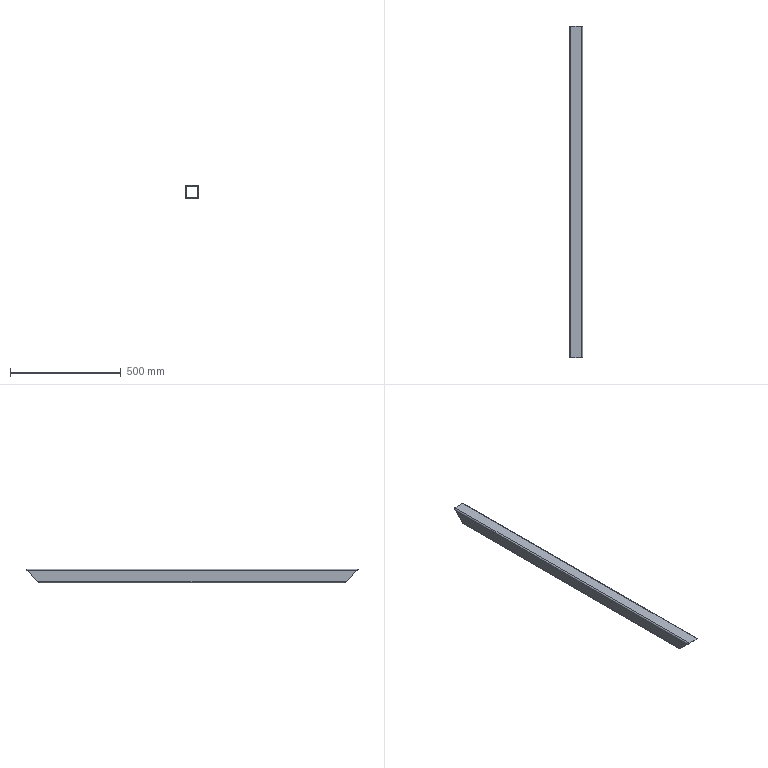Part | STEP file | Positioning_id1334_x_t | 1 solid | 14 faces | box 60 x 1500 x 60 mm | volume 1539500 mm3 | plane 10 | cylinder 4 | commonest cylinder face diameters 12 x4
STEP:
#1=CARTESIAN_POINT('',(0.,0.,0.));
#2=DIRECTION('',(0.,0.,1.));
#3=DIRECTION('',(1.,0.,0.));
#4=AXIS2_PLACEMENT_3D('',#1,#2,#3);
#5=CARTESIAN_POINT('',(-1086.002,695.,477.466));
#6=VERTEX_POINT('',#5);
#7=CARTESIAN_POINT('',(-1086.002,745.,527.466));
#8=VERTEX_POINT('',#7);
#9=CARTESIAN_POINT('',(-1086.002,695.,477.466));
#10=DIRECTION('',(0.,0.7071,0.7071));
#11=VECTOR('',#10,1.);
#12=LINE('',#9,#11);
#13=CARTESIAN_POINT('',(-1091.002,696.,478.466));
#14=DIRECTION('',(0.,-0.7071,0.7071));
#15=DIRECTION('',(0.,0.7071,0.7071));
#16=AXIS2_PLACEMENT_3D('',#13,#14,#15);
#17=PLANE('',#16);
#18=CARTESIAN_POINT('',(-1.414,-5.));
#19=DIRECTION('',(1.,0.));
#20=VECTOR('',#19,1.);
#21=LINE('',#18,#20);
#22=(GEOMETRIC_REPRESENTATION_CONTEXT(2)PARAMETRIC_REPRESENTATION_CONTEXT()REPRESENTATION_CONTEXT('',''));
#23=DEFINITIONAL_REPRESENTATION('',(#21),#22);
#24=PCURVE('',#17,#23);
#25=CARTESIAN_POINT('',(-1086.002,-375.,527.466));
#26=DIRECTION('',(-1.,0.,0.));
#27=DIRECTION('',(0.,0.,-1.));
#28=AXIS2_PLACEMENT_3D('',#25,#26,#27);
#29=PLANE('',#28);
#30=CARTESIAN_POINT('',(50.,-1070.));
#31=DIRECTION('',(-0.7071,-0.7071));
#32=VECTOR('',#31,1.);
#33=LINE('',#30,#32);
#34=(GEOMETRIC_REPRESENTATION_CONTEXT(2)PARAMETRIC_REPRESENTATION_CONTEXT()REPRESENTATION_CONTEXT('',''));
#35=DEFINITIONAL_REPRESENTATION('',(#33),#34);
#36=PCURVE('',#29,#35);
#37=SURFACE_CURVE('',#12,(#24,#36),.PCURVE_S1.);
#38=EDGE_CURVE('',#6,#8,#37,.T.);
#39=ORIENTED_EDGE('',*,*,#38,.F.);
#40=CARTESIAN_POINT('',(-1036.002,695.,477.466));
#41=VERTEX_POINT('',#40);
#42=CARTESIAN_POINT('',(-1036.002,695.,477.466));
#43=DIRECTION('',(-1.,0.,0.));
#44=VECTOR('',#43,1.);
#45=LINE('',#42,#44);
#46=CARTESIAN_POINT('',(-1.414,-55.));
#47=DIRECTION('',(0.,1.));
#48=VECTOR('',#47,1.);
#49=LINE('',#46,#48);
#50=(GEOMETRIC_REPRESENTATION_CONTEXT(2)PARAMETRIC_REPRESENTATION_CONTEXT()REPRESENTATION_CONTEXT('',''));
#51=DEFINITIONAL_REPRESENTATION('',(#49),#50);
#52=PCURVE('',#17,#51);
#53=CARTESIAN_POINT('',(-1061.002,-375.,477.466));
#54=DIRECTION('',(0.,0.,-1.));
#55=DIRECTION('',(1.,0.,0.));
#56=AXIS2_PLACEMENT_3D('',#53,#54,#55);
#57=PLANE('',#56);
#58=CARTESIAN_POINT('',(25.,-1070.));
#59=DIRECTION('',(-1.,0.));
#60=VECTOR('',#59,1.);
#61=LINE('',#58,#60);
#62=(GEOMETRIC_REPRESENTATION_CONTEXT(2)PARAMETRIC_REPRESENTATION_CONTEXT()REPRESENTATION_CONTEXT('',''));
#63=DEFINITIONAL_REPRESENTATION('',(#61),#62);
#64=PCURVE('',#57,#63);
#65=SURFACE_CURVE('',#45,(#52,#64),.PCURVE_S1.);
#66=EDGE_CURVE('',#41,#6,#65,.T.);
#67=ORIENTED_EDGE('',*,*,#66,.F.);
#68=CARTESIAN_POINT('',(-1036.002,745.,527.466));
#69=VERTEX_POINT('',#68);
#70=CARTESIAN_POINT('',(-1036.002,745.,527.466));
#71=DIRECTION('',(0.,-0.7071,-0.7071));
#72=VECTOR('',#71,1.);
#73=LINE('',#70,#72);
#74=CARTESIAN_POINT('',(69.296,-55.));
#75=DIRECTION('',(-1.,0.));
#76=VECTOR('',#75,1.);
#77=LINE('',#74,#76);
#78=(GEOMETRIC_REPRESENTATION_CONTEXT(2)PARAMETRIC_REPRESENTATION_CONTEXT()REPRESENTATION_CONTEXT('',''));
#79=DEFINITIONAL_REPRESENTATION('',(#77),#78);
#80=PCURVE('',#17,#79);
#81=CARTESIAN_POINT('',(-1036.002,-375.,527.466));
#82=DIRECTION('',(1.,0.,0.));
#83=DIRECTION('',(0.,0.,1.));
#84=AXIS2_PLACEMENT_3D('',#81,#82,#83);
#85=PLANE('',#84);
#86=CARTESIAN_POINT('',(0.,-1120.));
#87=DIRECTION('',(-0.7071,0.7071));
#88=VECTOR('',#87,1.);
#89=LINE('',#86,#88);
#90=(GEOMETRIC_REPRESENTATION_CONTEXT(2)PARAMETRIC_REPRESENTATION_CONTEXT()REPRESENTATION_CONTEXT('',''));
#91=DEFINITIONAL_REPRESENTATION('',(#89),#90);
#92=PCURVE('',#85,#91);
#93=SURFACE_CURVE('',#73,(#80,#92),.PCURVE_S1.);
#94=EDGE_CURVE('',#69,#41,#93,.T.);
#95=ORIENTED_EDGE('',*,*,#94,.F.);
#96=CARTESIAN_POINT('',(-1086.002,745.,527.466));
#97=DIRECTION('',(1.,0.,0.));
#98=VECTOR('',#97,1.);
#99=LINE('',#96,#98);
#100=CARTESIAN_POINT('',(69.296,-5.));
#101=DIRECTION('',(0.,-1.));
#102=VECTOR('',#101,1.);
#103=LINE('',#100,#102);
#104=(GEOMETRIC_REPRESENTATION_CONTEXT(2)PARAMETRIC_REPRESENTATION_CONTEXT()REPRESENTATION_CONTEXT('',''));
#105=DEFINITIONAL_REPRESENTATION('',(#103),#104);
#106=PCURVE('',#17,#105);
#107=CARTESIAN_POINT('',(-1061.002,-375.,527.466));
#108=DIRECTION('',(0.,0.,1.));
#109=DIRECTION('',(-1.,0.,0.));
#110=AXIS2_PLACEMENT_3D('',#107,#108,#109);
#111=PLANE('',#110);
#112=CARTESIAN_POINT('',(25.,-1120.));
#113=DIRECTION('',(-1.,0.));
#114=VECTOR('',#113,1.);
#115=LINE('',#112,#114);
#116=(GEOMETRIC_REPRESENTATION_CONTEXT(2)PARAMETRIC_REPRESENTATION_CONTEXT()REPRESENTATION_CONTEXT('',''));
#117=DEFINITIONAL_REPRESENTATION('',(#115),#116);
#118=PCURVE('',#111,#117);
#119=SURFACE_CURVE('',#99,(#106,#118),.PCURVE_S1.);
#120=EDGE_CURVE('',#8,#69,#119,.T.);
#121=ORIENTED_EDGE('',*,*,#120,.F.);
#122=EDGE_LOOP('',(#39,#67,#95,#121));
#123=FACE_BOUND('',#122,.T.);
#124=CARTESIAN_POINT('',(-1091.002,744.,526.466));
#125=VERTEX_POINT('',#124);
#126=CARTESIAN_POINT('',(-1085.002,750.,532.466));
#127=VERTEX_POINT('',#126);
#128=CARTESIAN_POINT('',(-1085.002,744.,526.466));
#129=DIRECTION('',(0.,0.7071,-0.7071));
#130=DIRECTION('',(0.,-0.7071,-0.7071));
#131=AXIS2_PLACEMENT_3D('',#128,#129,#130);
#132=ELLIPSE('',#131,8.485,6.);
#133=CARTESIAN_POINT('',(59.397,-6.));
#134=CARTESIAN_POINT('',(59.397,4.392));
#135=CARTESIAN_POINT('',(72.125,-0.8038));
#136=CARTESIAN_POINT('',(84.853,-6.));
#137=CARTESIAN_POINT('',(72.125,-11.196));
#138=CARTESIAN_POINT('',(59.397,-16.392));
#139=CARTESIAN_POINT('',(59.397,-6.));
#140=(BOUNDED_CURVE()B_SPLINE_CURVE(2,(#133,#134,#135,#136,#137,#138,#139),.UNSPECIFIED.,.T.,.F.)B_SPLINE_CURVE_WITH_KNOTS((1,2,2,2,2,1),(-2.094,0.,2.094,4.189,6.283,8.378),.UNSPECIFIED.)CURVE()GEOMETRIC_REPRESENTATION_ITEM()RATIONAL_B_SPLINE_CURVE((1.,0.5,1.,0.5,1.,0.5,1.))REPRESENTATION_ITEM(''));
#141=(GEOMETRIC_REPRESENTATION_CONTEXT(2)PARAMETRIC_REPRESENTATION_CONTEXT()REPRESENTATION_CONTEXT('',''));
#142=DEFINITIONAL_REPRESENTATION('',(#140),#141);
#143=PCURVE('',#17,#142);
#144=CARTESIAN_POINT('',(-1085.002,-375.,526.466));
#145=DIRECTION('',(0.,-1.,0.));
#146=DIRECTION('',(0.,0.,-1.));
#147=AXIS2_PLACEMENT_3D('',#144,#145,#146);
#148=CYLINDRICAL_SURFACE('',#147,6.);
#149=CARTESIAN_POINT('',(4.712,-1119.));
#150=CARTESIAN_POINT('',(4.689,-1119.143));
#151=CARTESIAN_POINT('',(4.641,-1119.428));
#152=CARTESIAN_POINT('',(4.57,-1119.855));
#153=CARTESIAN_POINT('',(4.498,-1120.276));
#154=CARTESIAN_POINT('',(4.427,-1120.692));
#155=CARTESIAN_POINT('',(4.355,-1121.099));
#156=CARTESIAN_POINT('',(4.284,-1121.495));
#157=CARTESIAN_POINT('',(4.213,-1121.878));
#158=CARTESIAN_POINT('',(4.141,-1122.247));
#159=CARTESIAN_POINT('',(4.07,-1122.599));
#160=CARTESIAN_POINT('',(3.998,-1122.933));
#161=CARTESIAN_POINT('',(3.927,-1123.246));
#162=CARTESIAN_POINT('',(3.856,-1123.538));
#163=CARTESIAN_POINT('',(3.784,-1123.807));
#164=CARTESIAN_POINT('',(3.713,-1124.052));
#165=CARTESIAN_POINT('',(3.641,-1124.271));
#166=CARTESIAN_POINT('',(3.57,-1124.462));
#167=CARTESIAN_POINT('',(3.499,-1124.626));
#168=CARTESIAN_POINT('',(3.427,-1124.762));
#169=CARTESIAN_POINT('',(3.356,-1124.868));
#170=CARTESIAN_POINT('',(3.284,-1124.944));
#171=CARTESIAN_POINT('',(3.213,-1124.99));
#172=CARTESIAN_POINT('',(3.165,-1125.));
#173=CARTESIAN_POINT('',(3.142,-1125.));
#174=B_SPLINE_CURVE_WITH_KNOTS('',3,(#149,#150,#151,#152,#153,#154,#155,#156,#157,#158,#159,#160,#161,#162,#163,#164,#165,#166,#167,#168,#169,#170,#171,#172,#173),.UNSPECIFIED.,.F.,.F.,(4,1,1,1,1,1,1,1,1,1,1,1,1,1,1,1,1,1,1,1,1,1,4),(1.571,1.642,1.714,1.785,1.856,1.928,1.999,2.071,2.142,2.213,2.285,2.356,2.428,2.499,2.57,2.642,2.713,2.785,2.856,2.927,2.999,3.07,3.142),.QUASI_UNIFORM_KNOTS.);
#175=(GEOMETRIC_REPRESENTATION_CONTEXT(2)PARAMETRIC_REPRESENTATION_CONTEXT()REPRESENTATION_CONTEXT('',''));
#176=DEFINITIONAL_REPRESENTATION('',(#174),#175);
#177=PCURVE('',#148,#176);
#178=SURFACE_CURVE('',#132,(#143,#177),.PCURVE_S1.);
#179=EDGE_CURVE('',#125,#127,#178,.T.);
#180=ORIENTED_EDGE('',*,*,#179,.T.);
#181=CARTESIAN_POINT('',(-1037.002,750.,532.466));
#182=VERTEX_POINT('',#181);
#183=CARTESIAN_POINT('',(-1085.002,750.,532.466));
#184=DIRECTION('',(1.,0.,0.));
#185=VECTOR('',#184,1.);
#186=LINE('',#183,#185);
#187=CARTESIAN_POINT('',(76.368,-6.));
#188=DIRECTION('',(0.,-1.));
#189=VECTOR('',#188,1.);
#190=LINE('',#187,#189);
#191=(GEOMETRIC_REPRESENTATION_CONTEXT(2)PARAMETRIC_REPRESENTATION_CONTEXT()REPRESENTATION_CONTEXT('',''));
#192=DEFINITIONAL_REPRESENTATION('',(#190),#191);
#193=PCURVE('',#17,#192);
#194=CARTESIAN_POINT('',(-1061.002,-375.,532.466));
#195=DIRECTION('',(0.,0.,1.));
#196=DIRECTION('',(-1.,0.,0.));
#197=AXIS2_PLACEMENT_3D('',#194,#195,#196);
#198=PLANE('',#197);
#199=CARTESIAN_POINT('',(24.,-1125.));
#200=DIRECTION('',(-1.,0.));
#201=VECTOR('',#200,1.);
#202=LINE('',#199,#201);
#203=(GEOMETRIC_REPRESENTATION_CONTEXT(2)PARAMETRIC_REPRESENTATION_CONTEXT()REPRESENTATION_CONTEXT('',''));
#204=DEFINITIONAL_REPRESENTATION('',(#202),#203);
#205=PCURVE('',#198,#204);
#206=SURFACE_CURVE('',#186,(#193,#205),.PCURVE_S1.);
#207=EDGE_CURVE('',#127,#182,#206,.T.);
#208=ORIENTED_EDGE('',*,*,#207,.T.);
#209=CARTESIAN_POINT('',(-1031.002,744.,526.466));
#210=VERTEX_POINT('',#209);
#211=CARTESIAN_POINT('',(-1037.002,744.,526.466));
#212=DIRECTION('',(0.,0.7071,-0.7071));
#213=DIRECTION('',(0.,0.7071,0.7071));
#214=AXIS2_PLACEMENT_3D('',#211,#212,#213);
#215=ELLIPSE('',#214,8.485,6.);
#216=CARTESIAN_POINT('',(76.368,-54.));
#217=CARTESIAN_POINT('',(76.368,-64.392));
#218=CARTESIAN_POINT('',(63.64,-59.196));
#219=CARTESIAN_POINT('',(50.912,-54.));
#220=CARTESIAN_POINT('',(63.64,-48.804));
#221=CARTESIAN_POINT('',(76.368,-43.608));
#222=CARTESIAN_POINT('',(76.368,-54.));
#223=(BOUNDED_CURVE()B_SPLINE_CURVE(2,(#216,#217,#218,#219,#220,#221,#222),.UNSPECIFIED.,.T.,.F.)B_SPLINE_CURVE_WITH_KNOTS((1,2,2,2,2,1),(-2.094,0.,2.094,4.189,6.283,8.378),.UNSPECIFIED.)CURVE()GEOMETRIC_REPRESENTATION_ITEM()RATIONAL_B_SPLINE_CURVE((1.,0.5,1.,0.5,1.,0.5,1.))REPRESENTATION_ITEM(''));
#224=(GEOMETRIC_REPRESENTATION_CONTEXT(2)PARAMETRIC_REPRESENTATION_CONTEXT()REPRESENTATION_CONTEXT('',''));
#225=DEFINITIONAL_REPRESENTATION('',(#223),#224);
#226=PCURVE('',#17,#225);
#227=CARTESIAN_POINT('',(-1037.002,-375.,526.466));
#228=DIRECTION('',(0.,1.,0.));
#229=DIRECTION('',(0.,0.,1.));
#230=AXIS2_PLACEMENT_3D('',#227,#228,#229);
#231=CYLINDRICAL_SURFACE('',#230,6.);
#232=CARTESIAN_POINT('',(0.,1125.));
#233=CARTESIAN_POINT('',(0.0238,1125.));
#234=CARTESIAN_POINT('',(0.0714,1124.99));
#235=CARTESIAN_POINT('',(0.1428,1124.944));
#236=CARTESIAN_POINT('',(0.2142,1124.868));
#237=CARTESIAN_POINT('',(0.2856,1124.762));
#238=CARTESIAN_POINT('',(0.357,1124.626));
#239=CARTESIAN_POINT('',(0.4284,1124.462));
#240=CARTESIAN_POINT('',(0.4998,1124.271));
#241=CARTESIAN_POINT('',(0.5712,1124.052));
#242=CARTESIAN_POINT('',(0.6426,1123.807));
#243=CARTESIAN_POINT('',(0.714,1123.538));
#244=CARTESIAN_POINT('',(0.7854,1123.246));
#245=CARTESIAN_POINT('',(0.8568,1122.933));
#246=CARTESIAN_POINT('',(0.9282,1122.599));
#247=CARTESIAN_POINT('',(0.9996,1122.247));
#248=CARTESIAN_POINT('',(1.071,1121.878));
#249=CARTESIAN_POINT('',(1.142,1121.495));
#250=CARTESIAN_POINT('',(1.214,1121.099));
#251=CARTESIAN_POINT('',(1.285,1120.692));
#252=CARTESIAN_POINT('',(1.357,1120.276));
#253=CARTESIAN_POINT('',(1.428,1119.855));
#254=CARTESIAN_POINT('',(1.499,1119.428));
#255=CARTESIAN_POINT('',(1.547,1119.143));
#256=CARTESIAN_POINT('',(1.571,1119.));
#257=B_SPLINE_CURVE_WITH_KNOTS('',3,(#232,#233,#234,#235,#236,#237,#238,#239,#240,#241,#242,#243,#244,#245,#246,#247,#248,#249,#250,#251,#252,#253,#254,#255,#256),.UNSPECIFIED.,.F.,.F.,(4,1,1,1,1,1,1,1,1,1,1,1,1,1,1,1,1,1,1,1,1,1,4),(0.,0.0714,0.1428,0.2142,0.2856,0.357,0.4284,0.4998,0.5712,0.6426,0.714,0.7854,0.8568,0.9282,0.9996,1.071,1.142,1.214,1.285,1.357,1.428,1.499,1.571),.QUASI_UNIFORM_KNOTS.);
#258=(GEOMETRIC_REPRESENTATION_CONTEXT(2)PARAMETRIC_REPRESENTATION_CONTEXT()REPRESENTATION_CONTEXT('',''));
#259=DEFINITIONAL_REPRESENTATION('',(#257),#258);
#260=PCURVE('',#231,#259);
#261=SURFACE_CURVE('',#215,(#226,#260),.PCURVE_S1.);
#262=EDGE_CURVE('',#182,#210,#261,.T.);
#263=ORIENTED_EDGE('',*,*,#262,.T.);
#264=CARTESIAN_POINT('',(-1031.002,696.,478.466));
#265=VERTEX_POINT('',#264);
#266=CARTESIAN_POINT('',(-1031.002,744.,526.466));
#267=DIRECTION('',(0.,-0.7071,-0.7071));
#268=VECTOR('',#267,1.);
#269=LINE('',#266,#268);
#270=CARTESIAN_POINT('',(67.882,-60.));
#271=DIRECTION('',(-1.,0.));
#272=VECTOR('',#271,1.);
#273=LINE('',#270,#272);
#274=(GEOMETRIC_REPRESENTATION_CONTEXT(2)PARAMETRIC_REPRESENTATION_CONTEXT()REPRESENTATION_CONTEXT('',''));
#275=DEFINITIONAL_REPRESENTATION('',(#273),#274);
#276=PCURVE('',#17,#275);
#277=CARTESIAN_POINT('',(-1031.002,-375.,532.466));
#278=DIRECTION('',(1.,0.,0.));
#279=DIRECTION('',(0.,0.,1.));
#280=AXIS2_PLACEMENT_3D('',#277,#278,#279);
#281=PLANE('',#280);
#282=CARTESIAN_POINT('',(-6.,-1119.));
#283=DIRECTION('',(-0.7071,0.7071));
#284=VECTOR('',#283,1.);
#285=LINE('',#282,#284);
#286=(GEOMETRIC_REPRESENTATION_CONTEXT(2)PARAMETRIC_REPRESENTATION_CONTEXT()REPRESENTATION_CONTEXT('',''));
#287=DEFINITIONAL_REPRESENTATION('',(#285),#286);
#288=PCURVE('',#281,#287);
#289=SURFACE_CURVE('',#269,(#276,#288),.PCURVE_S1.);
#290=EDGE_CURVE('',#210,#265,#289,.T.);
#291=ORIENTED_EDGE('',*,*,#290,.T.);
#292=CARTESIAN_POINT('',(-1037.002,690.,472.466));
#293=VERTEX_POINT('',#292);
#294=CARTESIAN_POINT('',(-1037.002,696.,478.466));
#295=DIRECTION('',(0.,0.7071,-0.7071));
#296=DIRECTION('',(0.,-0.7071,-0.7071));
#297=AXIS2_PLACEMENT_3D('',#294,#295,#296);
#298=ELLIPSE('',#297,8.485,6.);
#299=CARTESIAN_POINT('',(-8.485,-54.));
#300=CARTESIAN_POINT('',(-8.485,-43.608));
#301=CARTESIAN_POINT('',(4.243,-48.804));
#302=CARTESIAN_POINT('',(16.971,-54.));
#303=CARTESIAN_POINT('',(4.243,-59.196));
#304=CARTESIAN_POINT('',(-8.485,-64.392));
#305=CARTESIAN_POINT('',(-8.485,-54.));
#306=(BOUNDED_CURVE()B_SPLINE_CURVE(2,(#299,#300,#301,#302,#303,#304,#305),.UNSPECIFIED.,.T.,.F.)B_SPLINE_CURVE_WITH_KNOTS((1,2,2,2,2,1),(-2.094,0.,2.094,4.189,6.283,8.378),.UNSPECIFIED.)CURVE()GEOMETRIC_REPRESENTATION_ITEM()RATIONAL_B_SPLINE_CURVE((1.,0.5,1.,0.5,1.,0.5,1.))REPRESENTATION_ITEM(''));
#307=(GEOMETRIC_REPRESENTATION_CONTEXT(2)PARAMETRIC_REPRESENTATION_CONTEXT()REPRESENTATION_CONTEXT('',''));
#308=DEFINITIONAL_REPRESENTATION('',(#306),#307);
#309=PCURVE('',#17,#308);
#310=CARTESIAN_POINT('',(-1037.002,-375.,478.466));
#311=DIRECTION('',(0.,-1.,0.));
#312=DIRECTION('',(0.,0.,-1.));
#313=AXIS2_PLACEMENT_3D('',#310,#311,#312);
#314=CYLINDRICAL_SURFACE('',#313,6.);
#315=CARTESIAN_POINT('',(1.571,-1071.));
#316=CARTESIAN_POINT('',(1.547,-1070.857));
#317=CARTESIAN_POINT('',(1.499,-1070.572));
#318=CARTESIAN_POINT('',(1.428,-1070.145));
#319=CARTESIAN_POINT('',(1.357,-1069.724));
#320=CARTESIAN_POINT('',(1.285,-1069.308));
#321=CARTESIAN_POINT('',(1.214,-1068.901));
#322=CARTESIAN_POINT('',(1.142,-1068.505));
#323=CARTESIAN_POINT('',(1.071,-1068.122));
#324=CARTESIAN_POINT('',(0.9996,-1067.753));
#325=CARTESIAN_POINT('',(0.9282,-1067.401));
#326=CARTESIAN_POINT('',(0.8568,-1067.067));
#327=CARTESIAN_POINT('',(0.7854,-1066.754));
#328=CARTESIAN_POINT('',(0.714,-1066.462));
#329=CARTESIAN_POINT('',(0.6426,-1066.193));
#330=CARTESIAN_POINT('',(0.5712,-1065.948));
#331=CARTESIAN_POINT('',(0.4998,-1065.729));
#332=CARTESIAN_POINT('',(0.4284,-1065.538));
#333=CARTESIAN_POINT('',(0.357,-1065.374));
#334=CARTESIAN_POINT('',(0.2856,-1065.238));
#335=CARTESIAN_POINT('',(0.2142,-1065.132));
#336=CARTESIAN_POINT('',(0.1428,-1065.056));
#337=CARTESIAN_POINT('',(0.0714,-1065.01));
#338=CARTESIAN_POINT('',(0.0238,-1065.));
#339=CARTESIAN_POINT('',(0.,-1065.));
#340=B_SPLINE_CURVE_WITH_KNOTS('',3,(#315,#316,#317,#318,#319,#320,#321,#322,#323,#324,#325,#326,#327,#328,#329,#330,#331,#332,#333,#334,#335,#336,#337,#338,#339),.UNSPECIFIED.,.F.,.F.,(4,1,1,1,1,1,1,1,1,1,1,1,1,1,1,1,1,1,1,1,1,1,4),(4.712,4.784,4.855,4.927,4.998,5.069,5.141,5.212,5.284,5.355,5.426,5.498,5.569,5.641,5.712,5.783,5.855,5.926,5.998,6.069,6.14,6.212,6.283),.QUASI_UNIFORM_KNOTS.);
#341=(GEOMETRIC_REPRESENTATION_CONTEXT(2)PARAMETRIC_REPRESENTATION_CONTEXT()REPRESENTATION_CONTEXT('',''));
#342=DEFINITIONAL_REPRESENTATION('',(#340),#341);
#343=PCURVE('',#314,#342);
#344=SURFACE_CURVE('',#298,(#309,#343),.PCURVE_S1.);
#345=EDGE_CURVE('',#265,#293,#344,.T.);
#346=ORIENTED_EDGE('',*,*,#345,.T.);
#347=CARTESIAN_POINT('',(-1085.002,690.,472.466));
#348=VERTEX_POINT('',#347);
#349=CARTESIAN_POINT('',(-1037.002,690.,472.466));
#350=DIRECTION('',(-1.,0.,0.));
#351=VECTOR('',#350,1.);
#352=LINE('',#349,#351);
#353=CARTESIAN_POINT('',(-8.485,-54.));
#354=DIRECTION('',(0.,1.));
#355=VECTOR('',#354,1.);
#356=LINE('',#353,#355);
#357=(GEOMETRIC_REPRESENTATION_CONTEXT(2)PARAMETRIC_REPRESENTATION_CONTEXT()REPRESENTATION_CONTEXT('',''));
#358=DEFINITIONAL_REPRESENTATION('',(#356),#357);
#359=PCURVE('',#17,#358);
#360=CARTESIAN_POINT('',(-1061.002,-375.,472.466));
#361=DIRECTION('',(0.,0.,-1.));
#362=DIRECTION('',(1.,0.,0.));
#363=AXIS2_PLACEMENT_3D('',#360,#361,#362);
#364=PLANE('',#363);
#365=CARTESIAN_POINT('',(24.,-1065.));
#366=DIRECTION('',(-1.,0.));
#367=VECTOR('',#366,1.);
#368=LINE('',#365,#367);
#369=(GEOMETRIC_REPRESENTATION_CONTEXT(2)PARAMETRIC_REPRESENTATION_CONTEXT()REPRESENTATION_CONTEXT('',''));
#370=DEFINITIONAL_REPRESENTATION('',(#368),#369);
#371=PCURVE('',#364,#370);
#372=SURFACE_CURVE('',#352,(#359,#371),.PCURVE_S1.);
#373=EDGE_CURVE('',#293,#348,#372,.T.);
#374=ORIENTED_EDGE('',*,*,#373,.T.);
#375=CARTESIAN_POINT('',(-1091.002,696.,478.466));
#376=VERTEX_POINT('',#375);
#377=CARTESIAN_POINT('',(-1085.002,696.,478.466));
#378=DIRECTION('',(0.,0.7071,-0.7071));
#379=DIRECTION('',(0.,0.7071,0.7071));
#380=AXIS2_PLACEMENT_3D('',#377,#378,#379);
#381=ELLIPSE('',#380,8.485,6.);
#382=CARTESIAN_POINT('',(8.485,-6.));
#383=CARTESIAN_POINT('',(8.485,-16.392));
#384=CARTESIAN_POINT('',(-4.243,-11.196));
#385=CARTESIAN_POINT('',(-16.971,-6.));
#386=CARTESIAN_POINT('',(-4.243,-0.8038));
#387=CARTESIAN_POINT('',(8.485,4.392));
#388=CARTESIAN_POINT('',(8.485,-6.));
#389=(BOUNDED_CURVE()B_SPLINE_CURVE(2,(#382,#383,#384,#385,#386,#387,#388),.UNSPECIFIED.,.T.,.F.)B_SPLINE_CURVE_WITH_KNOTS((1,2,2,2,2,1),(-2.094,0.,2.094,4.189,6.283,8.378),.UNSPECIFIED.)CURVE()GEOMETRIC_REPRESENTATION_ITEM()RATIONAL_B_SPLINE_CURVE((1.,0.5,1.,0.5,1.,0.5,1.))REPRESENTATION_ITEM(''));
#390=(GEOMETRIC_REPRESENTATION_CONTEXT(2)PARAMETRIC_REPRESENTATION_CONTEXT()REPRESENTATION_CONTEXT('',''));
#391=DEFINITIONAL_REPRESENTATION('',(#389),#390);
#392=PCURVE('',#17,#391);
#393=CARTESIAN_POINT('',(-1085.002,-375.,478.466));
#394=DIRECTION('',(0.,1.,0.));
#395=DIRECTION('',(0.,0.,1.));
#396=AXIS2_PLACEMENT_3D('',#393,#394,#395);
#397=CYLINDRICAL_SURFACE('',#396,6.);
#398=CARTESIAN_POINT('',(3.142,1065.));
#399=CARTESIAN_POINT('',(3.165,1065.));
#400=CARTESIAN_POINT('',(3.213,1065.01));
#401=CARTESIAN_POINT('',(3.284,1065.056));
#402=CARTESIAN_POINT('',(3.356,1065.132));
#403=CARTESIAN_POINT('',(3.427,1065.238));
#404=CARTESIAN_POINT('',(3.499,1065.374));
#405=CARTESIAN_POINT('',(3.57,1065.538));
#406=CARTESIAN_POINT('',(3.641,1065.729));
#407=CARTESIAN_POINT('',(3.713,1065.948));
#408=CARTESIAN_POINT('',(3.784,1066.193));
#409=CARTESIAN_POINT('',(3.856,1066.462));
#410=CARTESIAN_POINT('',(3.927,1066.754));
#411=CARTESIAN_POINT('',(3.998,1067.067));
#412=CARTESIAN_POINT('',(4.07,1067.401));
#413=CARTESIAN_POINT('',(4.141,1067.753));
#414=CARTESIAN_POINT('',(4.213,1068.122));
#415=CARTESIAN_POINT('',(4.284,1068.505));
#416=CARTESIAN_POINT('',(4.355,1068.901));
#417=CARTESIAN_POINT('',(4.427,1069.308));
#418=CARTESIAN_POINT('',(4.498,1069.724));
#419=CARTESIAN_POINT('',(4.57,1070.145));
#420=CARTESIAN_POINT('',(4.641,1070.572));
#421=CARTESIAN_POINT('',(4.689,1070.857));
#422=CARTESIAN_POINT('',(4.712,1071.));
#423=B_SPLINE_CURVE_WITH_KNOTS('',3,(#398,#399,#400,#401,#402,#403,#404,#405,#406,#407,#408,#409,#410,#411,#412,#413,#414,#415,#416,#417,#418,#419,#420,#421,#422),.UNSPECIFIED.,.F.,.F.,(4,1,1,1,1,1,1,1,1,1,1,1,1,1,1,1,1,1,1,1,1,1,4),(3.142,3.213,3.284,3.356,3.427,3.499,3.57,3.641,3.713,3.784,3.856,3.927,3.998,4.07,4.141,4.213,4.284,4.355,4.427,4.498,4.57,4.641,4.712),.QUASI_UNIFORM_KNOTS.);
#424=(GEOMETRIC_REPRESENTATION_CONTEXT(2)PARAMETRIC_REPRESENTATION_CONTEXT()REPRESENTATION_CONTEXT('',''));
#425=DEFINITIONAL_REPRESENTATION('',(#423),#424);
#426=PCURVE('',#397,#425);
#427=SURFACE_CURVE('',#381,(#392,#426),.PCURVE_S1.);
#428=EDGE_CURVE('',#348,#376,#427,.T.);
#429=ORIENTED_EDGE('',*,*,#428,.T.);
#430=CARTESIAN_POINT('',(-1091.002,696.,478.466));
#431=DIRECTION('',(0.,0.7071,0.7071));
#432=VECTOR('',#431,1.);
#433=LINE('',#430,#432);
#434=CARTESIAN_POINT('',(0.,0.));
#435=DIRECTION('',(1.,0.));
#436=VECTOR('',#435,1.);
#437=LINE('',#434,#436);
#438=(GEOMETRIC_REPRESENTATION_CONTEXT(2)PARAMETRIC_REPRESENTATION_CONTEXT()REPRESENTATION_CONTEXT('',''));
#439=DEFINITIONAL_REPRESENTATION('',(#437),#438);
#440=PCURVE('',#17,#439);
#441=CARTESIAN_POINT('',(-1091.002,-375.,532.466));
#442=DIRECTION('',(-1.,0.,0.));
#443=DIRECTION('',(0.,0.,-1.));
#444=AXIS2_PLACEMENT_3D('',#441,#442,#443);
#445=PLANE('',#444);
#446=CARTESIAN_POINT('',(54.,-1071.));
#447=DIRECTION('',(-0.7071,-0.7071));
#448=VECTOR('',#447,1.);
#449=LINE('',#446,#448);
#450=(GEOMETRIC_REPRESENTATION_CONTEXT(2)PARAMETRIC_REPRESENTATION_CONTEXT()REPRESENTATION_CONTEXT('',''));
#451=DEFINITIONAL_REPRESENTATION('',(#449),#450);
#452=PCURVE('',#445,#451);
#453=SURFACE_CURVE('',#433,(#440,#452),.PCURVE_S1.);
#454=EDGE_CURVE('',#376,#125,#453,.T.);
#455=ORIENTED_EDGE('',*,*,#454,.T.);
#456=EDGE_LOOP('',(#180,#208,#263,#291,#346,#374,#429,#455));
#457=FACE_BOUND('',#456,.T.);
#458=ADVANCED_FACE('',(#123,#457),#17,.F.);
#459=CARTESIAN_POINT('',(-1036.002,-695.,477.466));
#460=VERTEX_POINT('',#459);
#461=CARTESIAN_POINT('',(-1086.002,-695.,477.466));
#462=VERTEX_POINT('',#461);
#463=CARTESIAN_POINT('',(-1036.002,-695.,477.466));
#464=DIRECTION('',(-1.,0.,0.));
#465=VECTOR('',#464,1.);
#466=LINE('',#463,#465);
#467=CARTESIAN_POINT('',(-1091.002,-696.,478.466));
#468=DIRECTION('',(0.,-0.7071,-0.7071));
#469=DIRECTION('',(0.,-0.7071,0.7071));
#470=AXIS2_PLACEMENT_3D('',#467,#468,#469);
#471=PLANE('',#470);
#472=CARTESIAN_POINT('',(-1.414,-55.));
#473=DIRECTION('',(0.,1.));
#474=VECTOR('',#473,1.);
#475=LINE('',#472,#474);
#476=(GEOMETRIC_REPRESENTATION_CONTEXT(2)PARAMETRIC_REPRESENTATION_CONTEXT()REPRESENTATION_CONTEXT('',''));
#477=DEFINITIONAL_REPRESENTATION('',(#475),#476);
#478=PCURVE('',#471,#477);
#479=CARTESIAN_POINT('',(25.,320.));
#480=DIRECTION('',(-1.,0.));
#481=VECTOR('',#480,1.);
#482=LINE('',#479,#481);
#483=(GEOMETRIC_REPRESENTATION_CONTEXT(2)PARAMETRIC_REPRESENTATION_CONTEXT()REPRESENTATION_CONTEXT('',''));
#484=DEFINITIONAL_REPRESENTATION('',(#482),#483);
#485=PCURVE('',#57,#484);
#486=SURFACE_CURVE('',#466,(#478,#485),.PCURVE_S1.);
#487=EDGE_CURVE('',#460,#462,#486,.T.);
#488=ORIENTED_EDGE('',*,*,#487,.T.);
#489=CARTESIAN_POINT('',(-1086.002,-745.,527.466));
#490=VERTEX_POINT('',#489);
#491=CARTESIAN_POINT('',(-1086.002,-695.,477.466));
#492=DIRECTION('',(0.,-0.7071,0.7071));
#493=VECTOR('',#492,1.);
#494=LINE('',#491,#493);
#495=CARTESIAN_POINT('',(-1.414,-5.));
#496=DIRECTION('',(1.,0.));
#497=VECTOR('',#496,1.);
#498=LINE('',#495,#497);
#499=(GEOMETRIC_REPRESENTATION_CONTEXT(2)PARAMETRIC_REPRESENTATION_CONTEXT()REPRESENTATION_CONTEXT('',''));
#500=DEFINITIONAL_REPRESENTATION('',(#498),#499);
#501=PCURVE('',#471,#500);
#502=CARTESIAN_POINT('',(50.,320.));
#503=DIRECTION('',(-0.7071,0.7071));
#504=VECTOR('',#503,1.);
#505=LINE('',#502,#504);
#506=(GEOMETRIC_REPRESENTATION_CONTEXT(2)PARAMETRIC_REPRESENTATION_CONTEXT()REPRESENTATION_CONTEXT('',''));
#507=DEFINITIONAL_REPRESENTATION('',(#505),#506);
#508=PCURVE('',#29,#507);
#509=SURFACE_CURVE('',#494,(#501,#508),.PCURVE_S1.);
#510=EDGE_CURVE('',#462,#490,#509,.T.);
#511=ORIENTED_EDGE('',*,*,#510,.T.);
#512=CARTESIAN_POINT('',(-1036.002,-745.,527.466));
#513=VERTEX_POINT('',#512);
#514=CARTESIAN_POINT('',(-1086.002,-745.,527.466));
#515=DIRECTION('',(1.,0.,0.));
#516=VECTOR('',#515,1.);
#517=LINE('',#514,#516);
#518=CARTESIAN_POINT('',(69.296,-5.));
#519=DIRECTION('',(0.,-1.));
#520=VECTOR('',#519,1.);
#521=LINE('',#518,#520);
#522=(GEOMETRIC_REPRESENTATION_CONTEXT(2)PARAMETRIC_REPRESENTATION_CONTEXT()REPRESENTATION_CONTEXT('',''));
#523=DEFINITIONAL_REPRESENTATION('',(#521),#522);
#524=PCURVE('',#471,#523);
#525=CARTESIAN_POINT('',(25.,370.));
#526=DIRECTION('',(-1.,0.));
#527=VECTOR('',#526,1.);
#528=LINE('',#525,#527);
#529=(GEOMETRIC_REPRESENTATION_CONTEXT(2)PARAMETRIC_REPRESENTATION_CONTEXT()REPRESENTATION_CONTEXT('',''));
#530=DEFINITIONAL_REPRESENTATION('',(#528),#529);
#531=PCURVE('',#111,#530);
#532=SURFACE_CURVE('',#517,(#524,#531),.PCURVE_S1.);
#533=EDGE_CURVE('',#490,#513,#532,.T.);
#534=ORIENTED_EDGE('',*,*,#533,.T.);
#535=CARTESIAN_POINT('',(-1036.002,-745.,527.466));
#536=DIRECTION('',(0.,0.7071,-0.7071));
#537=VECTOR('',#536,1.);
#538=LINE('',#535,#537);
#539=CARTESIAN_POINT('',(69.296,-55.));
#540=DIRECTION('',(-1.,0.));
#541=VECTOR('',#540,1.);
#542=LINE('',#539,#541);
#543=(GEOMETRIC_REPRESENTATION_CONTEXT(2)PARAMETRIC_REPRESENTATION_CONTEXT()REPRESENTATION_CONTEXT('',''));
#544=DEFINITIONAL_REPRESENTATION('',(#542),#543);
#545=PCURVE('',#471,#544);
#546=CARTESIAN_POINT('',(0.,370.));
#547=DIRECTION('',(-0.7071,-0.7071));
#548=VECTOR('',#547,1.);
#549=LINE('',#546,#548);
#550=(GEOMETRIC_REPRESENTATION_CONTEXT(2)PARAMETRIC_REPRESENTATION_CONTEXT()REPRESENTATION_CONTEXT('',''));
#551=DEFINITIONAL_REPRESENTATION('',(#549),#550);
#552=PCURVE('',#85,#551);
#553=SURFACE_CURVE('',#538,(#545,#552),.PCURVE_S1.);
#554=EDGE_CURVE('',#513,#460,#553,.T.);
#555=ORIENTED_EDGE('',*,*,#554,.T.);
#556=EDGE_LOOP('',(#488,#511,#534,#555));
#557=FACE_BOUND('',#556,.T.);
#558=CARTESIAN_POINT('',(-1085.002,-750.,532.466));
#559=VERTEX_POINT('',#558);
#560=CARTESIAN_POINT('',(-1037.002,-750.,532.466));
#561=VERTEX_POINT('',#560);
#562=CARTESIAN_POINT('',(-1085.002,-750.,532.466));
#563=DIRECTION('',(1.,0.,0.));
#564=VECTOR('',#563,1.);
#565=LINE('',#562,#564);
#566=CARTESIAN_POINT('',(76.368,-6.));
#567=DIRECTION('',(0.,-1.));
#568=VECTOR('',#567,1.);
#569=LINE('',#566,#568);
#570=(GEOMETRIC_REPRESENTATION_CONTEXT(2)PARAMETRIC_REPRESENTATION_CONTEXT()REPRESENTATION_CONTEXT('',''));
#571=DEFINITIONAL_REPRESENTATION('',(#569),#570);
#572=PCURVE('',#471,#571);
#573=CARTESIAN_POINT('',(24.,375.));
#574=DIRECTION('',(-1.,0.));
#575=VECTOR('',#574,1.);
#576=LINE('',#573,#575);
#577=(GEOMETRIC_REPRESENTATION_CONTEXT(2)PARAMETRIC_REPRESENTATION_CONTEXT()REPRESENTATION_CONTEXT('',''));
#578=DEFINITIONAL_REPRESENTATION('',(#576),#577);
#579=PCURVE('',#198,#578);
#580=SURFACE_CURVE('',#565,(#572,#579),.PCURVE_S1.);
#581=EDGE_CURVE('',#559,#561,#580,.T.);
#582=ORIENTED_EDGE('',*,*,#581,.F.);
#583=CARTESIAN_POINT('',(-1091.002,-744.,526.466));
#584=VERTEX_POINT('',#583);
#585=CARTESIAN_POINT('',(-1085.002,-744.,526.466));
#586=DIRECTION('',(0.,0.7071,0.7071));
#587=DIRECTION('',(0.,-0.7071,0.7071));
#588=AXIS2_PLACEMENT_3D('',#585,#586,#587);
#589=ELLIPSE('',#588,8.485,6.);
#590=CARTESIAN_POINT('',(76.368,-6.));
#591=CARTESIAN_POINT('',(76.368,-16.392));
#592=CARTESIAN_POINT('',(63.64,-11.196));
#593=CARTESIAN_POINT('',(50.912,-6.));
#594=CARTESIAN_POINT('',(63.64,-0.8038));
#595=CARTESIAN_POINT('',(76.368,4.392));
#596=CARTESIAN_POINT('',(76.368,-6.));
#597=(BOUNDED_CURVE()B_SPLINE_CURVE(2,(#590,#591,#592,#593,#594,#595,#596),.UNSPECIFIED.,.T.,.F.)B_SPLINE_CURVE_WITH_KNOTS((1,2,2,2,2,1),(-2.094,0.,2.094,4.189,6.283,8.378),.UNSPECIFIED.)CURVE()GEOMETRIC_REPRESENTATION_ITEM()RATIONAL_B_SPLINE_CURVE((1.,0.5,1.,0.5,1.,0.5,1.))REPRESENTATION_ITEM(''));
#598=(GEOMETRIC_REPRESENTATION_CONTEXT(2)PARAMETRIC_REPRESENTATION_CONTEXT()REPRESENTATION_CONTEXT('',''));
#599=DEFINITIONAL_REPRESENTATION('',(#597),#598);
#600=PCURVE('',#471,#599);
#601=CARTESIAN_POINT('',(4.712,369.));
#602=CARTESIAN_POINT('',(4.689,369.143));
#603=CARTESIAN_POINT('',(4.641,369.428));
#604=CARTESIAN_POINT('',(4.57,369.855));
#605=CARTESIAN_POINT('',(4.498,370.276));
#606=CARTESIAN_POINT('',(4.427,370.692));
#607=CARTESIAN_POINT('',(4.355,371.099));
#608=CARTESIAN_POINT('',(4.284,371.495));
#609=CARTESIAN_POINT('',(4.213,371.878));
#610=CARTESIAN_POINT('',(4.141,372.247));
#611=CARTESIAN_POINT('',(4.07,372.599));
#612=CARTESIAN_POINT('',(3.998,372.933));
#613=CARTESIAN_POINT('',(3.927,373.246));
#614=CARTESIAN_POINT('',(3.856,373.538));
#615=CARTESIAN_POINT('',(3.784,373.807));
#616=CARTESIAN_POINT('',(3.713,374.052));
#617=CARTESIAN_POINT('',(3.641,374.271));
#618=CARTESIAN_POINT('',(3.57,374.462));
#619=CARTESIAN_POINT('',(3.499,374.626));
#620=CARTESIAN_POINT('',(3.427,374.762));
#621=CARTESIAN_POINT('',(3.356,374.868));
#622=CARTESIAN_POINT('',(3.284,374.944));
#623=CARTESIAN_POINT('',(3.213,374.99));
#624=CARTESIAN_POINT('',(3.165,375.));
#625=CARTESIAN_POINT('',(3.142,375.));
#626=B_SPLINE_CURVE_WITH_KNOTS('',3,(#601,#602,#603,#604,#605,#606,#607,#608,#609,#610,#611,#612,#613,#614,#615,#616,#617,#618,#619,#620,#621,#622,#623,#624,#625),.UNSPECIFIED.,.F.,.F.,(4,1,1,1,1,1,1,1,1,1,1,1,1,1,1,1,1,1,1,1,1,1,4),(4.712,4.784,4.855,4.927,4.998,5.069,5.141,5.212,5.284,5.355,5.426,5.498,5.569,5.641,5.712,5.783,5.855,5.926,5.998,6.069,6.14,6.212,6.283),.QUASI_UNIFORM_KNOTS.);
#627=(GEOMETRIC_REPRESENTATION_CONTEXT(2)PARAMETRIC_REPRESENTATION_CONTEXT()REPRESENTATION_CONTEXT('',''));
#628=DEFINITIONAL_REPRESENTATION('',(#626),#627);
#629=PCURVE('',#148,#628);
#630=SURFACE_CURVE('',#589,(#600,#629),.PCURVE_S1.);
#631=EDGE_CURVE('',#584,#559,#630,.T.);
#632=ORIENTED_EDGE('',*,*,#631,.F.);
#633=CARTESIAN_POINT('',(-1091.002,-696.,478.466));
#634=VERTEX_POINT('',#633);
#635=CARTESIAN_POINT('',(-1091.002,-696.,478.466));
#636=DIRECTION('',(0.,-0.7071,0.7071));
#637=VECTOR('',#636,1.);
#638=LINE('',#635,#637);
#639=CARTESIAN_POINT('',(0.,0.));
#640=DIRECTION('',(1.,0.));
#641=VECTOR('',#640,1.);
#642=LINE('',#639,#641);
#643=(GEOMETRIC_REPRESENTATION_CONTEXT(2)PARAMETRIC_REPRESENTATION_CONTEXT()REPRESENTATION_CONTEXT('',''));
#644=DEFINITIONAL_REPRESENTATION('',(#642),#643);
#645=PCURVE('',#471,#644);
#646=CARTESIAN_POINT('',(54.,321.));
#647=DIRECTION('',(-0.7071,0.7071));
#648=VECTOR('',#647,1.);
#649=LINE('',#646,#648);
#650=(GEOMETRIC_REPRESENTATION_CONTEXT(2)PARAMETRIC_REPRESENTATION_CONTEXT()REPRESENTATION_CONTEXT('',''));
#651=DEFINITIONAL_REPRESENTATION('',(#649),#650);
#652=PCURVE('',#445,#651);
#653=SURFACE_CURVE('',#638,(#645,#652),.PCURVE_S1.);
#654=EDGE_CURVE('',#634,#584,#653,.T.);
#655=ORIENTED_EDGE('',*,*,#654,.F.);
#656=CARTESIAN_POINT('',(-1085.002,-690.,472.466));
#657=VERTEX_POINT('',#656);
#658=CARTESIAN_POINT('',(-1085.002,-696.,478.466));
#659=DIRECTION('',(0.,0.7071,0.7071));
#660=DIRECTION('',(0.,0.7071,-0.7071));
#661=AXIS2_PLACEMENT_3D('',#658,#659,#660);
#662=ELLIPSE('',#661,8.485,6.);
#663=CARTESIAN_POINT('',(-8.485,-6.));
#664=CARTESIAN_POINT('',(-8.485,4.392));
#665=CARTESIAN_POINT('',(4.243,-0.8038));
#666=CARTESIAN_POINT('',(16.971,-6.));
#667=CARTESIAN_POINT('',(4.243,-11.196));
#668=CARTESIAN_POINT('',(-8.485,-16.392));
#669=CARTESIAN_POINT('',(-8.485,-6.));
#670=(BOUNDED_CURVE()B_SPLINE_CURVE(2,(#663,#664,#665,#666,#667,#668,#669),.UNSPECIFIED.,.T.,.F.)B_SPLINE_CURVE_WITH_KNOTS((1,2,2,2,2,1),(-2.094,0.,2.094,4.189,6.283,8.378),.UNSPECIFIED.)CURVE()GEOMETRIC_REPRESENTATION_ITEM()RATIONAL_B_SPLINE_CURVE((1.,0.5,1.,0.5,1.,0.5,1.))REPRESENTATION_ITEM(''));
#671=(GEOMETRIC_REPRESENTATION_CONTEXT(2)PARAMETRIC_REPRESENTATION_CONTEXT()REPRESENTATION_CONTEXT('',''));
#672=DEFINITIONAL_REPRESENTATION('',(#670),#671);
#673=PCURVE('',#471,#672);
#674=CARTESIAN_POINT('',(3.142,-315.));
#675=CARTESIAN_POINT('',(3.165,-315.));
#676=CARTESIAN_POINT('',(3.213,-315.01));
#677=CARTESIAN_POINT('',(3.284,-315.056));
#678=CARTESIAN_POINT('',(3.356,-315.132));
#679=CARTESIAN_POINT('',(3.427,-315.238));
#680=CARTESIAN_POINT('',(3.499,-315.374));
#681=CARTESIAN_POINT('',(3.57,-315.538));
#682=CARTESIAN_POINT('',(3.641,-315.729));
#683=CARTESIAN_POINT('',(3.713,-315.948));
#684=CARTESIAN_POINT('',(3.784,-316.193));
#685=CARTESIAN_POINT('',(3.856,-316.462));
#686=CARTESIAN_POINT('',(3.927,-316.754));
#687=CARTESIAN_POINT('',(3.998,-317.067));
#688=CARTESIAN_POINT('',(4.07,-317.401));
#689=CARTESIAN_POINT('',(4.141,-317.753));
#690=CARTESIAN_POINT('',(4.213,-318.122));
#691=CARTESIAN_POINT('',(4.284,-318.505));
#692=CARTESIAN_POINT('',(4.355,-318.901));
#693=CARTESIAN_POINT('',(4.427,-319.308));
#694=CARTESIAN_POINT('',(4.498,-319.724));
#695=CARTESIAN_POINT('',(4.57,-320.145));
#696=CARTESIAN_POINT('',(4.641,-320.572));
#697=CARTESIAN_POINT('',(4.689,-320.857));
#698=CARTESIAN_POINT('',(4.712,-321.));
#699=B_SPLINE_CURVE_WITH_KNOTS('',3,(#674,#675,#676,#677,#678,#679,#680,#681,#682,#683,#684,#685,#686,#687,#688,#689,#690,#691,#692,#693,#694,#695,#696,#697,#698),.UNSPECIFIED.,.F.,.F.,(4,1,1,1,1,1,1,1,1,1,1,1,1,1,1,1,1,1,1,1,1,1,4),(0.,0.0714,0.1428,0.2142,0.2856,0.357,0.4284,0.4998,0.5712,0.6426,0.714,0.7854,0.8568,0.9282,0.9996,1.071,1.142,1.214,1.285,1.357,1.428,1.499,1.571),.QUASI_UNIFORM_KNOTS.);
#700=(GEOMETRIC_REPRESENTATION_CONTEXT(2)PARAMETRIC_REPRESENTATION_CONTEXT()REPRESENTATION_CONTEXT('',''));
#701=DEFINITIONAL_REPRESENTATION('',(#699),#700);
#702=PCURVE('',#397,#701);
#703=SURFACE_CURVE('',#662,(#673,#702),.PCURVE_S1.);
#704=EDGE_CURVE('',#657,#634,#703,.T.);
#705=ORIENTED_EDGE('',*,*,#704,.F.);
#706=CARTESIAN_POINT('',(-1037.002,-690.,472.466));
#707=VERTEX_POINT('',#706);
#708=CARTESIAN_POINT('',(-1037.002,-690.,472.466));
#709=DIRECTION('',(-1.,0.,0.));
#710=VECTOR('',#709,1.);
#711=LINE('',#708,#710);
#712=CARTESIAN_POINT('',(-8.485,-54.));
#713=DIRECTION('',(0.,1.));
#714=VECTOR('',#713,1.);
#715=LINE('',#712,#714);
#716=(GEOMETRIC_REPRESENTATION_CONTEXT(2)PARAMETRIC_REPRESENTATION_CONTEXT()REPRESENTATION_CONTEXT('',''));
#717=DEFINITIONAL_REPRESENTATION('',(#715),#716);
#718=PCURVE('',#471,#717);
#719=CARTESIAN_POINT('',(24.,315.));
#720=DIRECTION('',(-1.,0.));
#721=VECTOR('',#720,1.);
#722=LINE('',#719,#721);
#723=(GEOMETRIC_REPRESENTATION_CONTEXT(2)PARAMETRIC_REPRESENTATION_CONTEXT()REPRESENTATION_CONTEXT('',''));
#724=DEFINITIONAL_REPRESENTATION('',(#722),#723);
#725=PCURVE('',#364,#724);
#726=SURFACE_CURVE('',#711,(#718,#725),.PCURVE_S1.);
#727=EDGE_CURVE('',#707,#657,#726,.T.);
#728=ORIENTED_EDGE('',*,*,#727,.F.);
#729=CARTESIAN_POINT('',(-1031.002,-696.,478.466));
#730=VERTEX_POINT('',#729);
#731=CARTESIAN_POINT('',(-1037.002,-696.,478.466));
#732=DIRECTION('',(0.,0.7071,0.7071));
#733=DIRECTION('',(0.,-0.7071,0.7071));
#734=AXIS2_PLACEMENT_3D('',#731,#732,#733);
#735=ELLIPSE('',#734,8.485,6.);
#736=CARTESIAN_POINT('',(8.485,-54.));
#737=CARTESIAN_POINT('',(8.485,-64.392));
#738=CARTESIAN_POINT('',(-4.243,-59.196));
#739=CARTESIAN_POINT('',(-16.971,-54.));
#740=CARTESIAN_POINT('',(-4.243,-48.804));
#741=CARTESIAN_POINT('',(8.485,-43.608));
#742=CARTESIAN_POINT('',(8.485,-54.));
#743=(BOUNDED_CURVE()B_SPLINE_CURVE(2,(#736,#737,#738,#739,#740,#741,#742),.UNSPECIFIED.,.T.,.F.)B_SPLINE_CURVE_WITH_KNOTS((1,2,2,2,2,1),(-2.094,0.,2.094,4.189,6.283,8.378),.UNSPECIFIED.)CURVE()GEOMETRIC_REPRESENTATION_ITEM()RATIONAL_B_SPLINE_CURVE((1.,0.5,1.,0.5,1.,0.5,1.))REPRESENTATION_ITEM(''));
#744=(GEOMETRIC_REPRESENTATION_CONTEXT(2)PARAMETRIC_REPRESENTATION_CONTEXT()REPRESENTATION_CONTEXT('',''));
#745=DEFINITIONAL_REPRESENTATION('',(#743),#744);
#746=PCURVE('',#471,#745);
#747=CARTESIAN_POINT('',(1.571,321.));
#748=CARTESIAN_POINT('',(1.547,320.857));
#749=CARTESIAN_POINT('',(1.499,320.572));
#750=CARTESIAN_POINT('',(1.428,320.145));
#751=CARTESIAN_POINT('',(1.357,319.724));
#752=CARTESIAN_POINT('',(1.285,319.308));
#753=CARTESIAN_POINT('',(1.214,318.901));
#754=CARTESIAN_POINT('',(1.142,318.505));
#755=CARTESIAN_POINT('',(1.071,318.122));
#756=CARTESIAN_POINT('',(0.9996,317.753));
#757=CARTESIAN_POINT('',(0.9282,317.401));
#758=CARTESIAN_POINT('',(0.8568,317.067));
#759=CARTESIAN_POINT('',(0.7854,316.754));
#760=CARTESIAN_POINT('',(0.714,316.462));
#761=CARTESIAN_POINT('',(0.6426,316.193));
#762=CARTESIAN_POINT('',(0.5712,315.948));
#763=CARTESIAN_POINT('',(0.4998,315.729));
#764=CARTESIAN_POINT('',(0.4284,315.538));
#765=CARTESIAN_POINT('',(0.357,315.374));
#766=CARTESIAN_POINT('',(0.2856,315.238));
#767=CARTESIAN_POINT('',(0.2142,315.132));
#768=CARTESIAN_POINT('',(0.1428,315.056));
#769=CARTESIAN_POINT('',(0.0714,315.01));
#770=CARTESIAN_POINT('',(0.0238,315.));
#771=CARTESIAN_POINT('',(0.,315.));
#772=B_SPLINE_CURVE_WITH_KNOTS('',3,(#747,#748,#749,#750,#751,#752,#753,#754,#755,#756,#757,#758,#759,#760,#761,#762,#763,#764,#765,#766,#767,#768,#769,#770,#771),.UNSPECIFIED.,.F.,.F.,(4,1,1,1,1,1,1,1,1,1,1,1,1,1,1,1,1,1,1,1,1,1,4),(1.571,1.642,1.714,1.785,1.856,1.928,1.999,2.071,2.142,2.213,2.285,2.356,2.428,2.499,2.57,2.642,2.713,2.785,2.856,2.927,2.999,3.07,3.142),.QUASI_UNIFORM_KNOTS.);
#773=(GEOMETRIC_REPRESENTATION_CONTEXT(2)PARAMETRIC_REPRESENTATION_CONTEXT()REPRESENTATION_CONTEXT('',''));
#774=DEFINITIONAL_REPRESENTATION('',(#772),#773);
#775=PCURVE('',#314,#774);
#776=SURFACE_CURVE('',#735,(#746,#775),.PCURVE_S1.);
#777=EDGE_CURVE('',#730,#707,#776,.T.);
#778=ORIENTED_EDGE('',*,*,#777,.F.);
#779=CARTESIAN_POINT('',(-1031.002,-744.,526.466));
#780=VERTEX_POINT('',#779);
#781=CARTESIAN_POINT('',(-1031.002,-744.,526.466));
#782=DIRECTION('',(0.,0.7071,-0.7071));
#783=VECTOR('',#782,1.);
#784=LINE('',#781,#783);
#785=CARTESIAN_POINT('',(67.882,-60.));
#786=DIRECTION('',(-1.,0.));
#787=VECTOR('',#786,1.);
#788=LINE('',#785,#787);
#789=(GEOMETRIC_REPRESENTATION_CONTEXT(2)PARAMETRIC_REPRESENTATION_CONTEXT()REPRESENTATION_CONTEXT('',''));
#790=DEFINITIONAL_REPRESENTATION('',(#788),#789);
#791=PCURVE('',#471,#790);
#792=CARTESIAN_POINT('',(-6.,369.));
#793=DIRECTION('',(-0.7071,-0.7071));
#794=VECTOR('',#793,1.);
#795=LINE('',#792,#794);
#796=(GEOMETRIC_REPRESENTATION_CONTEXT(2)PARAMETRIC_REPRESENTATION_CONTEXT()REPRESENTATION_CONTEXT('',''));
#797=DEFINITIONAL_REPRESENTATION('',(#795),#796);
#798=PCURVE('',#281,#797);
#799=SURFACE_CURVE('',#784,(#791,#798),.PCURVE_S1.);
#800=EDGE_CURVE('',#780,#730,#799,.T.);
#801=ORIENTED_EDGE('',*,*,#800,.F.);
#802=CARTESIAN_POINT('',(-1037.002,-744.,526.466));
#803=DIRECTION('',(0.,0.7071,0.7071));
#804=DIRECTION('',(0.,0.7071,-0.7071));
#805=AXIS2_PLACEMENT_3D('',#802,#803,#804);
#806=ELLIPSE('',#805,8.485,6.);
#807=CARTESIAN_POINT('',(59.397,-54.));
#808=CARTESIAN_POINT('',(59.397,-43.608));
#809=CARTESIAN_POINT('',(72.125,-48.804));
#810=CARTESIAN_POINT('',(84.853,-54.));
#811=CARTESIAN_POINT('',(72.125,-59.196));
#812=CARTESIAN_POINT('',(59.397,-64.392));
#813=CARTESIAN_POINT('',(59.397,-54.));
#814=(BOUNDED_CURVE()B_SPLINE_CURVE(2,(#807,#808,#809,#810,#811,#812,#813),.UNSPECIFIED.,.T.,.F.)B_SPLINE_CURVE_WITH_KNOTS((1,2,2,2,2,1),(-2.094,0.,2.094,4.189,6.283,8.378),.UNSPECIFIED.)CURVE()GEOMETRIC_REPRESENTATION_ITEM()RATIONAL_B_SPLINE_CURVE((1.,0.5,1.,0.5,1.,0.5,1.))REPRESENTATION_ITEM(''));
#815=(GEOMETRIC_REPRESENTATION_CONTEXT(2)PARAMETRIC_REPRESENTATION_CONTEXT()REPRESENTATION_CONTEXT('',''));
#816=DEFINITIONAL_REPRESENTATION('',(#814),#815);
#817=PCURVE('',#471,#816);
#818=CARTESIAN_POINT('',(0.,-375.));
#819=CARTESIAN_POINT('',(0.0238,-375.));
#820=CARTESIAN_POINT('',(0.0714,-374.99));
#821=CARTESIAN_POINT('',(0.1428,-374.944));
#822=CARTESIAN_POINT('',(0.2142,-374.868));
#823=CARTESIAN_POINT('',(0.2856,-374.762));
#824=CARTESIAN_POINT('',(0.357,-374.626));
#825=CARTESIAN_POINT('',(0.4284,-374.462));
#826=CARTESIAN_POINT('',(0.4998,-374.271));
#827=CARTESIAN_POINT('',(0.5712,-374.052));
#828=CARTESIAN_POINT('',(0.6426,-373.807));
#829=CARTESIAN_POINT('',(0.714,-373.538));
#830=CARTESIAN_POINT('',(0.7854,-373.246));
#831=CARTESIAN_POINT('',(0.8568,-372.933));
#832=CARTESIAN_POINT('',(0.9282,-372.599));
#833=CARTESIAN_POINT('',(0.9996,-372.247));
#834=CARTESIAN_POINT('',(1.071,-371.878));
#835=CARTESIAN_POINT('',(1.142,-371.495));
#836=CARTESIAN_POINT('',(1.214,-371.099));
#837=CARTESIAN_POINT('',(1.285,-370.692));
#838=CARTESIAN_POINT('',(1.357,-370.276));
#839=CARTESIAN_POINT('',(1.428,-369.855));
#840=CARTESIAN_POINT('',(1.499,-369.428));
#841=CARTESIAN_POINT('',(1.547,-369.143));
#842=CARTESIAN_POINT('',(1.571,-369.));
#843=B_SPLINE_CURVE_WITH_KNOTS('',3,(#818,#819,#820,#821,#822,#823,#824,#825,#826,#827,#828,#829,#830,#831,#832,#833,#834,#835,#836,#837,#838,#839,#840,#841,#842),.UNSPECIFIED.,.F.,.F.,(4,1,1,1,1,1,1,1,1,1,1,1,1,1,1,1,1,1,1,1,1,1,4),(3.142,3.213,3.284,3.356,3.427,3.499,3.57,3.641,3.713,3.784,3.856,3.927,3.998,4.07,4.141,4.213,4.284,4.355,4.427,4.498,4.57,4.641,4.712),.QUASI_UNIFORM_KNOTS.);
#844=(GEOMETRIC_REPRESENTATION_CONTEXT(2)PARAMETRIC_REPRESENTATION_CONTEXT()REPRESENTATION_CONTEXT('',''));
#845=DEFINITIONAL_REPRESENTATION('',(#843),#844);
#846=PCURVE('',#231,#845);
#847=SURFACE_CURVE('',#806,(#817,#846),.PCURVE_S1.);
#848=EDGE_CURVE('',#561,#780,#847,.T.);
#849=ORIENTED_EDGE('',*,*,#848,.F.);
#850=EDGE_LOOP('',(#582,#632,#655,#705,#728,#778,#801,#849));
#851=FACE_BOUND('',#850,.T.);
#852=ADVANCED_FACE('',(#557,#851),#471,.T.);
#853=ORIENTED_EDGE('',*,*,#373,.F.);
#854=CARTESIAN_POINT('',(-1037.002,690.,472.466));
#855=DIRECTION('',(0.,-1.,0.));
#856=VECTOR('',#855,1.);
#857=LINE('',#854,#856);
#858=CARTESIAN_POINT('',(24.,-1065.));
#859=DIRECTION('',(0.,1.));
#860=VECTOR('',#859,1.);
#861=LINE('',#858,#860);
#862=(GEOMETRIC_REPRESENTATION_CONTEXT(2)PARAMETRIC_REPRESENTATION_CONTEXT()REPRESENTATION_CONTEXT('',''));
#863=DEFINITIONAL_REPRESENTATION('',(#861),#862);
#864=PCURVE('',#364,#863);
#865=CARTESIAN_POINT('',(0.,-1065.));
#866=DIRECTION('',(0.,1.));
#867=VECTOR('',#866,1.);
#868=LINE('',#865,#867);
#869=(GEOMETRIC_REPRESENTATION_CONTEXT(2)PARAMETRIC_REPRESENTATION_CONTEXT()REPRESENTATION_CONTEXT('',''));
#870=DEFINITIONAL_REPRESENTATION('',(#868),#869);
#871=PCURVE('',#314,#870);
#872=SURFACE_CURVE('',#857,(#864,#871),.PCURVE_S1.);
#873=EDGE_CURVE('',#293,#707,#872,.T.);
#874=ORIENTED_EDGE('',*,*,#873,.T.);
#875=ORIENTED_EDGE('',*,*,#727,.T.);
#876=CARTESIAN_POINT('',(-1085.002,-690.,472.466));
#877=DIRECTION('',(0.,1.,0.));
#878=VECTOR('',#877,1.);
#879=LINE('',#876,#878);
#880=CARTESIAN_POINT('',(-24.,315.));
#881=DIRECTION('',(0.,-1.));
#882=VECTOR('',#881,1.);
#883=LINE('',#880,#882);
#884=(GEOMETRIC_REPRESENTATION_CONTEXT(2)PARAMETRIC_REPRESENTATION_CONTEXT()REPRESENTATION_CONTEXT('',''));
#885=DEFINITIONAL_REPRESENTATION('',(#883),#884);
#886=PCURVE('',#364,#885);
#887=CARTESIAN_POINT('',(3.142,-315.));
#888=DIRECTION('',(0.,1.));
#889=VECTOR('',#888,1.);
#890=LINE('',#887,#889);
#891=(GEOMETRIC_REPRESENTATION_CONTEXT(2)PARAMETRIC_REPRESENTATION_CONTEXT()REPRESENTATION_CONTEXT('',''));
#892=DEFINITIONAL_REPRESENTATION('',(#890),#891);
#893=PCURVE('',#397,#892);
#894=SURFACE_CURVE('',#879,(#886,#893),.PCURVE_S1.);
#895=EDGE_CURVE('',#657,#348,#894,.T.);
#896=ORIENTED_EDGE('',*,*,#895,.T.);
#897=EDGE_LOOP('',(#853,#874,#875,#896));
#898=FACE_BOUND('',#897,.T.);
#899=ADVANCED_FACE('',(#898),#364,.T.);
#900=ORIENTED_EDGE('',*,*,#290,.F.);
#901=CARTESIAN_POINT('',(-1031.002,744.,526.466));
#902=DIRECTION('',(0.,-1.,0.));
#903=VECTOR('',#902,1.);
#904=LINE('',#901,#903);
#905=CARTESIAN_POINT('',(-6.,-1119.));
#906=DIRECTION('',(0.,1.));
#907=VECTOR('',#906,1.);
#908=LINE('',#905,#907);
#909=(GEOMETRIC_REPRESENTATION_CONTEXT(2)PARAMETRIC_REPRESENTATION_CONTEXT()REPRESENTATION_CONTEXT('',''));
#910=DEFINITIONAL_REPRESENTATION('',(#908),#909);
#911=PCURVE('',#281,#910);
#912=CARTESIAN_POINT('',(1.571,1119.));
#913=DIRECTION('',(0.,-1.));
#914=VECTOR('',#913,1.);
#915=LINE('',#912,#914);
#916=(GEOMETRIC_REPRESENTATION_CONTEXT(2)PARAMETRIC_REPRESENTATION_CONTEXT()REPRESENTATION_CONTEXT('',''));
#917=DEFINITIONAL_REPRESENTATION('',(#915),#916);
#918=PCURVE('',#231,#917);
#919=SURFACE_CURVE('',#904,(#911,#918),.PCURVE_S1.);
#920=EDGE_CURVE('',#210,#780,#919,.T.);
#921=ORIENTED_EDGE('',*,*,#920,.T.);
#922=ORIENTED_EDGE('',*,*,#800,.T.);
#923=CARTESIAN_POINT('',(-1031.002,-696.,478.466));
#924=DIRECTION('',(0.,1.,0.));
#925=VECTOR('',#924,1.);
#926=LINE('',#923,#925);
#927=CARTESIAN_POINT('',(-54.,321.));
#928=DIRECTION('',(0.,-1.));
#929=VECTOR('',#928,1.);
#930=LINE('',#927,#929);
#931=(GEOMETRIC_REPRESENTATION_CONTEXT(2)PARAMETRIC_REPRESENTATION_CONTEXT()REPRESENTATION_CONTEXT('',''));
#932=DEFINITIONAL_REPRESENTATION('',(#930),#931);
#933=PCURVE('',#281,#932);
#934=CARTESIAN_POINT('',(1.571,321.));
#935=DIRECTION('',(0.,-1.));
#936=VECTOR('',#935,1.);
#937=LINE('',#934,#936);
#938=(GEOMETRIC_REPRESENTATION_CONTEXT(2)PARAMETRIC_REPRESENTATION_CONTEXT()REPRESENTATION_CONTEXT('',''));
#939=DEFINITIONAL_REPRESENTATION('',(#937),#938);
#940=PCURVE('',#314,#939);
#941=SURFACE_CURVE('',#926,(#933,#940),.PCURVE_S1.);
#942=EDGE_CURVE('',#730,#265,#941,.T.);
#943=ORIENTED_EDGE('',*,*,#942,.T.);
#944=EDGE_LOOP('',(#900,#921,#922,#943));
#945=FACE_BOUND('',#944,.T.);
#946=ADVANCED_FACE('',(#945),#281,.T.);
#947=ORIENTED_EDGE('',*,*,#345,.F.);
#948=ORIENTED_EDGE('',*,*,#942,.F.);
#949=ORIENTED_EDGE('',*,*,#777,.T.);
#950=ORIENTED_EDGE('',*,*,#873,.F.);
#951=EDGE_LOOP('',(#947,#948,#949,#950));
#952=FACE_BOUND('',#951,.T.);
#953=ADVANCED_FACE('',(#952),#314,.T.);
#954=ORIENTED_EDGE('',*,*,#454,.F.);
#955=CARTESIAN_POINT('',(-1091.002,696.,478.466));
#956=DIRECTION('',(0.,-1.,0.));
#957=VECTOR('',#956,1.);
#958=LINE('',#955,#957);
#959=CARTESIAN_POINT('',(54.,-1071.));
#960=DIRECTION('',(0.,1.));
#961=VECTOR('',#960,1.);
#962=LINE('',#959,#961);
#963=(GEOMETRIC_REPRESENTATION_CONTEXT(2)PARAMETRIC_REPRESENTATION_CONTEXT()REPRESENTATION_CONTEXT('',''));
#964=DEFINITIONAL_REPRESENTATION('',(#962),#963);
#965=PCURVE('',#445,#964);
#966=CARTESIAN_POINT('',(4.712,1071.));
#967=DIRECTION('',(0.,-1.));
#968=VECTOR('',#967,1.);
#969=LINE('',#966,#968);
#970=(GEOMETRIC_REPRESENTATION_CONTEXT(2)PARAMETRIC_REPRESENTATION_CONTEXT()REPRESENTATION_CONTEXT('',''));
#971=DEFINITIONAL_REPRESENTATION('',(#969),#970);
#972=PCURVE('',#397,#971);
#973=SURFACE_CURVE('',#958,(#965,#972),.PCURVE_S1.);
#974=EDGE_CURVE('',#376,#634,#973,.T.);
#975=ORIENTED_EDGE('',*,*,#974,.T.);
#976=ORIENTED_EDGE('',*,*,#654,.T.);
#977=CARTESIAN_POINT('',(-1091.002,-744.,526.466));
#978=DIRECTION('',(0.,1.,0.));
#979=VECTOR('',#978,1.);
#980=LINE('',#977,#979);
#981=CARTESIAN_POINT('',(6.,369.));
#982=DIRECTION('',(0.,-1.));
#983=VECTOR('',#982,1.);
#984=LINE('',#981,#983);
#985=(GEOMETRIC_REPRESENTATION_CONTEXT(2)PARAMETRIC_REPRESENTATION_CONTEXT()REPRESENTATION_CONTEXT('',''));
#986=DEFINITIONAL_REPRESENTATION('',(#984),#985);
#987=PCURVE('',#445,#986);
#988=CARTESIAN_POINT('',(4.712,369.));
#989=DIRECTION('',(0.,-1.));
#990=VECTOR('',#989,1.);
#991=LINE('',#988,#990);
#992=(GEOMETRIC_REPRESENTATION_CONTEXT(2)PARAMETRIC_REPRESENTATION_CONTEXT()REPRESENTATION_CONTEXT('',''));
#993=DEFINITIONAL_REPRESENTATION('',(#991),#992);
#994=PCURVE('',#148,#993);
#995=SURFACE_CURVE('',#980,(#987,#994),.PCURVE_S1.);
#996=EDGE_CURVE('',#584,#125,#995,.T.);
#997=ORIENTED_EDGE('',*,*,#996,.T.);
#998=EDGE_LOOP('',(#954,#975,#976,#997));
#999=FACE_BOUND('',#998,.T.);
#1000=ADVANCED_FACE('',(#999),#445,.T.);
#1001=ORIENTED_EDGE('',*,*,#207,.F.);
#1002=CARTESIAN_POINT('',(-1085.002,750.,532.466));
#1003=DIRECTION('',(0.,-1.,0.));
#1004=VECTOR('',#1003,1.);
#1005=LINE('',#1002,#1004);
#1006=CARTESIAN_POINT('',(24.,-1125.));
#1007=DIRECTION('',(0.,1.));
#1008=VECTOR('',#1007,1.);
#1009=LINE('',#1006,#1008);
#1010=(GEOMETRIC_REPRESENTATION_CONTEXT(2)PARAMETRIC_REPRESENTATION_CONTEXT()REPRESENTATION_CONTEXT('',''));
#1011=DEFINITIONAL_REPRESENTATION('',(#1009),#1010);
#1012=PCURVE('',#198,#1011);
#1013=CARTESIAN_POINT('',(3.142,-1125.));
#1014=DIRECTION('',(0.,1.));
#1015=VECTOR('',#1014,1.);
#1016=LINE('',#1013,#1015);
#1017=(GEOMETRIC_REPRESENTATION_CONTEXT(2)PARAMETRIC_REPRESENTATION_CONTEXT()REPRESENTATION_CONTEXT('',''));
#1018=DEFINITIONAL_REPRESENTATION('',(#1016),#1017);
#1019=PCURVE('',#148,#1018);
#1020=SURFACE_CURVE('',#1005,(#1012,#1019),.PCURVE_S1.);
#1021=EDGE_CURVE('',#127,#559,#1020,.T.);
#1022=ORIENTED_EDGE('',*,*,#1021,.T.);
#1023=ORIENTED_EDGE('',*,*,#581,.T.);
#1024=CARTESIAN_POINT('',(-1037.002,-750.,532.466));
#1025=DIRECTION('',(0.,1.,0.));
#1026=VECTOR('',#1025,1.);
#1027=LINE('',#1024,#1026);
#1028=CARTESIAN_POINT('',(-24.,375.));
#1029=DIRECTION('',(0.,-1.));
#1030=VECTOR('',#1029,1.);
#1031=LINE('',#1028,#1030);
#1032=(GEOMETRIC_REPRESENTATION_CONTEXT(2)PARAMETRIC_REPRESENTATION_CONTEXT()REPRESENTATION_CONTEXT('',''));
#1033=DEFINITIONAL_REPRESENTATION('',(#1031),#1032);
#1034=PCURVE('',#198,#1033);
#1035=CARTESIAN_POINT('',(0.,-375.));
#1036=DIRECTION('',(0.,1.));
#1037=VECTOR('',#1036,1.);
#1038=LINE('',#1035,#1037);
#1039=(GEOMETRIC_REPRESENTATION_CONTEXT(2)PARAMETRIC_REPRESENTATION_CONTEXT()REPRESENTATION_CONTEXT('',''));
#1040=DEFINITIONAL_REPRESENTATION('',(#1038),#1039);
#1041=PCURVE('',#231,#1040);
#1042=SURFACE_CURVE('',#1027,(#1034,#1041),.PCURVE_S1.);
#1043=EDGE_CURVE('',#561,#182,#1042,.T.);
#1044=ORIENTED_EDGE('',*,*,#1043,.T.);
#1045=EDGE_LOOP('',(#1001,#1022,#1023,#1044));
#1046=FACE_BOUND('',#1045,.T.);
#1047=ADVANCED_FACE('',(#1046),#198,.T.);
#1048=ORIENTED_EDGE('',*,*,#262,.F.);
#1049=ORIENTED_EDGE('',*,*,#1043,.F.);
#1050=ORIENTED_EDGE('',*,*,#848,.T.);
#1051=ORIENTED_EDGE('',*,*,#920,.F.);
#1052=EDGE_LOOP('',(#1048,#1049,#1050,#1051));
#1053=FACE_BOUND('',#1052,.T.);
#1054=ADVANCED_FACE('',(#1053),#231,.T.);
#1055=ORIENTED_EDGE('',*,*,#179,.F.);
#1056=ORIENTED_EDGE('',*,*,#996,.F.);
#1057=ORIENTED_EDGE('',*,*,#631,.T.);
#1058=ORIENTED_EDGE('',*,*,#1021,.F.);
#1059=EDGE_LOOP('',(#1055,#1056,#1057,#1058));
#1060=FACE_BOUND('',#1059,.T.);
#1061=ADVANCED_FACE('',(#1060),#148,.T.);
#1062=ORIENTED_EDGE('',*,*,#428,.F.);
#1063=ORIENTED_EDGE('',*,*,#895,.F.);
#1064=ORIENTED_EDGE('',*,*,#704,.T.);
#1065=ORIENTED_EDGE('',*,*,#974,.F.);
#1066=EDGE_LOOP('',(#1062,#1063,#1064,#1065));
#1067=FACE_BOUND('',#1066,.T.);
#1068=ADVANCED_FACE('',(#1067),#397,.T.);
#1069=CARTESIAN_POINT('',(-1036.002,-695.,477.466));
#1070=DIRECTION('',(0.,1.,0.));
#1071=VECTOR('',#1070,1.);
#1072=LINE('',#1069,#1071);
#1073=CARTESIAN_POINT('',(25.,320.));
#1074=DIRECTION('',(0.,-1.));
#1075=VECTOR('',#1074,1.);
#1076=LINE('',#1073,#1075);
#1077=(GEOMETRIC_REPRESENTATION_CONTEXT(2)PARAMETRIC_REPRESENTATION_CONTEXT()REPRESENTATION_CONTEXT('',''));
#1078=DEFINITIONAL_REPRESENTATION('',(#1076),#1077);
#1079=PCURVE('',#57,#1078);
#1080=CARTESIAN_POINT('',(-50.,320.));
#1081=DIRECTION('',(0.,-1.));
#1082=VECTOR('',#1081,1.);
#1083=LINE('',#1080,#1082);
#1084=(GEOMETRIC_REPRESENTATION_CONTEXT(2)PARAMETRIC_REPRESENTATION_CONTEXT()REPRESENTATION_CONTEXT('',''));
#1085=DEFINITIONAL_REPRESENTATION('',(#1083),#1084);
#1086=PCURVE('',#85,#1085);
#1087=SURFACE_CURVE('',#1072,(#1079,#1086),.PCURVE_S1.);
#1088=EDGE_CURVE('',#460,#41,#1087,.T.);
#1089=ORIENTED_EDGE('',*,*,#1088,.T.);
#1090=ORIENTED_EDGE('',*,*,#66,.T.);
#1091=CARTESIAN_POINT('',(-1086.002,695.,477.466));
#1092=DIRECTION('',(0.,-1.,0.));
#1093=VECTOR('',#1092,1.);
#1094=LINE('',#1091,#1093);
#1095=CARTESIAN_POINT('',(-25.,-1070.));
#1096=DIRECTION('',(0.,1.));
#1097=VECTOR('',#1096,1.);
#1098=LINE('',#1095,#1097);
#1099=(GEOMETRIC_REPRESENTATION_CONTEXT(2)PARAMETRIC_REPRESENTATION_CONTEXT()REPRESENTATION_CONTEXT('',''));
#1100=DEFINITIONAL_REPRESENTATION('',(#1098),#1099);
#1101=PCURVE('',#57,#1100);
#1102=CARTESIAN_POINT('',(50.,-1070.));
#1103=DIRECTION('',(0.,1.));
#1104=VECTOR('',#1103,1.);
#1105=LINE('',#1102,#1104);
#1106=(GEOMETRIC_REPRESENTATION_CONTEXT(2)PARAMETRIC_REPRESENTATION_CONTEXT()REPRESENTATION_CONTEXT('',''));
#1107=DEFINITIONAL_REPRESENTATION('',(#1105),#1106);
#1108=PCURVE('',#29,#1107);
#1109=SURFACE_CURVE('',#1094,(#1101,#1108),.PCURVE_S1.);
#1110=EDGE_CURVE('',#6,#462,#1109,.T.);
#1111=ORIENTED_EDGE('',*,*,#1110,.T.);
#1112=ORIENTED_EDGE('',*,*,#487,.F.);
#1113=EDGE_LOOP('',(#1089,#1090,#1111,#1112));
#1114=FACE_BOUND('',#1113,.T.);
#1115=ADVANCED_FACE('',(#1114),#57,.F.);
#1116=CARTESIAN_POINT('',(-1036.002,745.,527.466));
#1117=DIRECTION('',(0.,-1.,0.));
#1118=VECTOR('',#1117,1.);
#1119=LINE('',#1116,#1118);
#1120=CARTESIAN_POINT('',(0.,-1120.));
#1121=DIRECTION('',(0.,1.));
#1122=VECTOR('',#1121,1.);
#1123=LINE('',#1120,#1122);
#1124=(GEOMETRIC_REPRESENTATION_CONTEXT(2)PARAMETRIC_REPRESENTATION_CONTEXT()REPRESENTATION_CONTEXT('',''));
#1125=DEFINITIONAL_REPRESENTATION('',(#1123),#1124);
#1126=PCURVE('',#85,#1125);
#1127=CARTESIAN_POINT('',(-25.,-1120.));
#1128=DIRECTION('',(0.,1.));
#1129=VECTOR('',#1128,1.);
#1130=LINE('',#1127,#1129);
#1131=(GEOMETRIC_REPRESENTATION_CONTEXT(2)PARAMETRIC_REPRESENTATION_CONTEXT()REPRESENTATION_CONTEXT('',''));
#1132=DEFINITIONAL_REPRESENTATION('',(#1130),#1131);
#1133=PCURVE('',#111,#1132);
#1134=SURFACE_CURVE('',#1119,(#1126,#1133),.PCURVE_S1.);
#1135=EDGE_CURVE('',#69,#513,#1134,.T.);
#1136=ORIENTED_EDGE('',*,*,#1135,.F.);
#1137=ORIENTED_EDGE('',*,*,#94,.T.);
#1138=ORIENTED_EDGE('',*,*,#1088,.F.);
#1139=ORIENTED_EDGE('',*,*,#554,.F.);
#1140=EDGE_LOOP('',(#1136,#1137,#1138,#1139));
#1141=FACE_BOUND('',#1140,.T.);
#1142=ADVANCED_FACE('',(#1141),#85,.F.);
#1143=CARTESIAN_POINT('',(-1086.002,-745.,527.466));
#1144=DIRECTION('',(0.,1.,0.));
#1145=VECTOR('',#1144,1.);
#1146=LINE('',#1143,#1145);
#1147=CARTESIAN_POINT('',(25.,370.));
#1148=DIRECTION('',(0.,-1.));
#1149=VECTOR('',#1148,1.);
#1150=LINE('',#1147,#1149);
#1151=(GEOMETRIC_REPRESENTATION_CONTEXT(2)PARAMETRIC_REPRESENTATION_CONTEXT()REPRESENTATION_CONTEXT('',''));
#1152=DEFINITIONAL_REPRESENTATION('',(#1150),#1151);
#1153=PCURVE('',#111,#1152);
#1154=CARTESIAN_POINT('',(0.,370.));
#1155=DIRECTION('',(0.,-1.));
#1156=VECTOR('',#1155,1.);
#1157=LINE('',#1154,#1156);
#1158=(GEOMETRIC_REPRESENTATION_CONTEXT(2)PARAMETRIC_REPRESENTATION_CONTEXT()REPRESENTATION_CONTEXT('',''));
#1159=DEFINITIONAL_REPRESENTATION('',(#1157),#1158);
#1160=PCURVE('',#29,#1159);
#1161=SURFACE_CURVE('',#1146,(#1153,#1160),.PCURVE_S1.);
#1162=EDGE_CURVE('',#490,#8,#1161,.T.);
#1163=ORIENTED_EDGE('',*,*,#1162,.T.);
#1164=ORIENTED_EDGE('',*,*,#120,.T.);
#1165=ORIENTED_EDGE('',*,*,#1135,.T.);
#1166=ORIENTED_EDGE('',*,*,#533,.F.);
#1167=EDGE_LOOP('',(#1163,#1164,#1165,#1166));
#1168=FACE_BOUND('',#1167,.T.);
#1169=ADVANCED_FACE('',(#1168),#111,.F.);
#1170=ORIENTED_EDGE('',*,*,#1110,.F.);
#1171=ORIENTED_EDGE('',*,*,#38,.T.);
#1172=ORIENTED_EDGE('',*,*,#1162,.F.);
#1173=ORIENTED_EDGE('',*,*,#510,.F.);
#1174=EDGE_LOOP('',(#1170,#1171,#1172,#1173));
#1175=FACE_BOUND('',#1174,.T.);
#1176=ADVANCED_FACE('',(#1175),#29,.F.);
#1177=CLOSED_SHELL('',(#458,#852,#899,#946,#953,#1000,#1047,#1054,#1061,#1068,#1115,#1142,#1169,#1176));
#1178=MANIFOLD_SOLID_BREP('',#1177);
#1179=(LENGTH_UNIT()NAMED_UNIT(*)SI_UNIT(.MILLI.,.METRE.));
#1180=UNCERTAINTY_MEASURE_WITH_UNIT(LENGTH_MEASURE(0.0000001),#1179,'','');
#1181=(NAMED_UNIT(*)PLANE_ANGLE_UNIT()SI_UNIT($,.RADIAN.));
#1182=(NAMED_UNIT(*)SI_UNIT($,.STERADIAN.)SOLID_ANGLE_UNIT());
#1183=(GEOMETRIC_REPRESENTATION_CONTEXT(3)GLOBAL_UNCERTAINTY_ASSIGNED_CONTEXT((#1180))GLOBAL_UNIT_ASSIGNED_CONTEXT((#1179,#1181,#1182))REPRESENTATION_CONTEXT('',''));
#1184=ADVANCED_BREP_SHAPE_REPRESENTATION('',(#4,#1178),#1183);